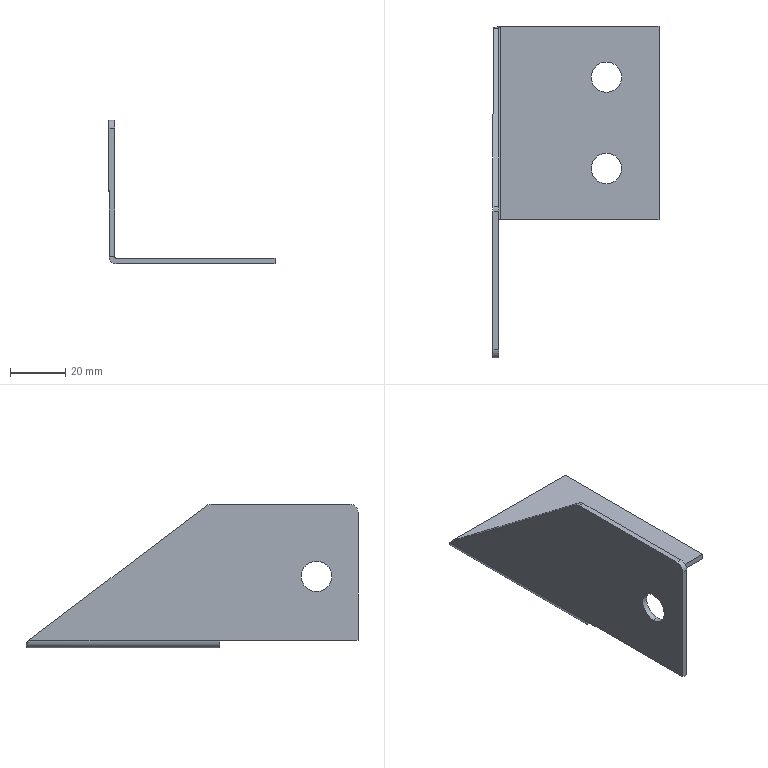Part | SolidWorks | features BaseBody 1 | 1 solid | 22 faces | box 60 x 120 x 52 mm | volume 16346 mm3 | plane 11 | cylinder 10 | spline 1 | commonest cylinder face diameters 11 x6 6 x2 1.473 x1 5.473 x1
STEP:
#1=CARTESIAN_POINT('',(-28.,-70.,18.368));
#2=VERTEX_POINT('',#1);
#3=CARTESIAN_POINT('',(-28.,-70.,29.368));
#4=VERTEX_POINT('',#3);
#5=CARTESIAN_POINT('',(-28.,-70.,23.868));
#6=DIRECTION('',(-1.,0.,0.));
#7=DIRECTION('',(0.,0.,1.));
#8=AXIS2_PLACEMENT_3D('',#5,#6,#7);
#9=CIRCLE('',#8,5.5);
#10=EDGE_CURVE('',#2,#4,#9,.T.);
#11=ORIENTED_EDGE('',*,*,#10,.F.);
#12=CARTESIAN_POINT('',(-30.,-70.,18.368));
#13=VERTEX_POINT('',#12);
#14=CARTESIAN_POINT('',(-20.,-70.,18.368));
#15=DIRECTION('',(-1.,0.,0.));
#16=VECTOR('',#15,1000.);
#17=LINE('',#14,#16);
#18=EDGE_CURVE('',#2,#13,#17,.T.);
#19=ORIENTED_EDGE('',*,*,#18,.T.);
#20=CARTESIAN_POINT('',(-30.,-70.,29.368));
#21=VERTEX_POINT('',#20);
#22=CARTESIAN_POINT('',(-30.,-70.,23.868));
#23=DIRECTION('',(1.,0.,0.));
#24=DIRECTION('',(0.,0.,1.));
#25=AXIS2_PLACEMENT_3D('',#22,#23,#24);
#26=CIRCLE('',#25,5.5);
#27=EDGE_CURVE('',#21,#13,#26,.T.);
#28=ORIENTED_EDGE('',*,*,#27,.F.);
#29=CARTESIAN_POINT('',(-20.,-70.,29.368));
#30=DIRECTION('',(-1.,0.,0.));
#31=VECTOR('',#30,1000.);
#32=LINE('',#29,#31);
#33=EDGE_CURVE('',#4,#21,#32,.T.);
#34=ORIENTED_EDGE('',*,*,#33,.F.);
#35=EDGE_LOOP('',(#11,#19,#28,#34));
#36=FACE_OUTER_BOUND('',#35,.T.);
#37=CARTESIAN_POINT('',(-20.,-70.,23.868));
#38=DIRECTION('',(-1.,0.,0.));
#39=DIRECTION('',(0.,0.,1.));
#40=AXIS2_PLACEMENT_3D('',#37,#38,#39);
#41=CYLINDRICAL_SURFACE('',#40,5.5);
#42=ADVANCED_FACE('',(#36),#41,.F.);
#43=CARTESIAN_POINT('',(5.5,16.5,-2.));
#44=VERTEX_POINT('',#43);
#45=CARTESIAN_POINT('',(16.5,16.5,-2.));
#46=VERTEX_POINT('',#45);
#47=CARTESIAN_POINT('',(11.,16.5,-2.));
#48=DIRECTION('',(0.,0.,1.));
#49=DIRECTION('',(1.,0.,0.));
#50=AXIS2_PLACEMENT_3D('',#47,#48,#49);
#51=CIRCLE('',#50,5.5);
#52=EDGE_CURVE('',#44,#46,#51,.T.);
#53=ORIENTED_EDGE('',*,*,#52,.F.);
#54=CARTESIAN_POINT('',(5.5,16.5,0.));
#55=VERTEX_POINT('',#54);
#56=CARTESIAN_POINT('',(5.5,16.5,-2.));
#57=DIRECTION('',(0.,0.,1.));
#58=VECTOR('',#57,1000.);
#59=LINE('',#56,#58);
#60=EDGE_CURVE('',#44,#55,#59,.T.);
#61=ORIENTED_EDGE('',*,*,#60,.T.);
#62=CARTESIAN_POINT('',(16.5,16.5,0.));
#63=VERTEX_POINT('',#62);
#64=CARTESIAN_POINT('',(11.,16.5,0.));
#65=DIRECTION('',(0.,0.,-1.));
#66=DIRECTION('',(1.,0.,0.));
#67=AXIS2_PLACEMENT_3D('',#64,#65,#66);
#68=CIRCLE('',#67,5.5);
#69=EDGE_CURVE('',#63,#55,#68,.T.);
#70=ORIENTED_EDGE('',*,*,#69,.F.);
#71=CARTESIAN_POINT('',(16.5,16.5,-2.));
#72=DIRECTION('',(0.,0.,1.));
#73=VECTOR('',#72,1000.);
#74=LINE('',#71,#73);
#75=EDGE_CURVE('',#46,#63,#74,.T.);
#76=ORIENTED_EDGE('',*,*,#75,.F.);
#77=EDGE_LOOP('',(#53,#61,#70,#76));
#78=FACE_OUTER_BOUND('',#77,.T.);
#79=CARTESIAN_POINT('',(11.,16.5,-2.));
#80=DIRECTION('',(0.,0.,1.));
#81=DIRECTION('',(1.,0.,0.));
#82=AXIS2_PLACEMENT_3D('',#79,#80,#81);
#83=CYLINDRICAL_SURFACE('',#82,5.5);
#84=ADVANCED_FACE('',(#78),#83,.F.);
#85=CARTESIAN_POINT('',(5.5,-16.5,-2.));
#86=VERTEX_POINT('',#85);
#87=CARTESIAN_POINT('',(16.5,-16.5,-2.));
#88=VERTEX_POINT('',#87);
#89=CARTESIAN_POINT('',(11.,-16.5,-2.));
#90=DIRECTION('',(0.,0.,1.));
#91=DIRECTION('',(1.,0.,0.));
#92=AXIS2_PLACEMENT_3D('',#89,#90,#91);
#93=CIRCLE('',#92,5.5);
#94=EDGE_CURVE('',#86,#88,#93,.T.);
#95=ORIENTED_EDGE('',*,*,#94,.F.);
#96=CARTESIAN_POINT('',(5.5,-16.5,0.));
#97=VERTEX_POINT('',#96);
#98=CARTESIAN_POINT('',(5.5,-16.5,-2.));
#99=DIRECTION('',(0.,0.,1.));
#100=VECTOR('',#99,1000.);
#101=LINE('',#98,#100);
#102=EDGE_CURVE('',#86,#97,#101,.T.);
#103=ORIENTED_EDGE('',*,*,#102,.T.);
#104=CARTESIAN_POINT('',(16.5,-16.5,0.));
#105=VERTEX_POINT('',#104);
#106=CARTESIAN_POINT('',(11.,-16.5,0.));
#107=DIRECTION('',(0.,0.,-1.));
#108=DIRECTION('',(1.,0.,0.));
#109=AXIS2_PLACEMENT_3D('',#106,#107,#108);
#110=CIRCLE('',#109,5.5);
#111=EDGE_CURVE('',#105,#97,#110,.T.);
#112=ORIENTED_EDGE('',*,*,#111,.F.);
#113=CARTESIAN_POINT('',(16.5,-16.5,-2.));
#114=DIRECTION('',(0.,0.,1.));
#115=VECTOR('',#114,1000.);
#116=LINE('',#113,#115);
#117=EDGE_CURVE('',#88,#105,#116,.T.);
#118=ORIENTED_EDGE('',*,*,#117,.F.);
#119=EDGE_LOOP('',(#95,#103,#112,#118));
#120=FACE_OUTER_BOUND('',#119,.T.);
#121=CARTESIAN_POINT('',(11.,-16.5,-2.));
#122=DIRECTION('',(0.,0.,1.));
#123=DIRECTION('',(1.,0.,0.));
#124=AXIS2_PLACEMENT_3D('',#121,#122,#123);
#125=CYLINDRICAL_SURFACE('',#124,5.5);
#126=ADVANCED_FACE('',(#120),#125,.F.);
#127=CARTESIAN_POINT('',(-30.,-82.,50.));
#128=VERTEX_POINT('',#127);
#129=CARTESIAN_POINT('',(-30.,-32.,50.));
#130=VERTEX_POINT('',#129);
#131=CARTESIAN_POINT('',(-30.,-32.,50.));
#132=DIRECTION('',(0.,1.,0.));
#133=VECTOR('',#132,1000.);
#134=LINE('',#131,#133);
#135=EDGE_CURVE('',#128,#130,#134,.T.);
#136=ORIENTED_EDGE('',*,*,#135,.T.);
#137=CARTESIAN_POINT('',(-30.,-30.188,49.391));
#138=VERTEX_POINT('',#137);
#139=CARTESIAN_POINT('',(-30.,-32.,47.));
#140=DIRECTION('',(-1.,0.,0.));
#141=DIRECTION('',(0.,0.,-1.));
#142=AXIS2_PLACEMENT_3D('',#139,#140,#141);
#143=CIRCLE('',#142,3.);
#144=EDGE_CURVE('',#130,#138,#143,.T.);
#145=ORIENTED_EDGE('',*,*,#144,.T.);
#146=CARTESIAN_POINT('',(-30.,34.028,0.7366));
#147=VERTEX_POINT('',#146);
#148=CARTESIAN_POINT('',(-30.,-30.188,49.391));
#149=DIRECTION('',(0.,0.7971,-0.6039));
#150=VECTOR('',#149,1000.);
#151=LINE('',#148,#150);
#152=EDGE_CURVE('',#138,#147,#151,.T.);
#153=ORIENTED_EDGE('',*,*,#152,.T.);
#154=CARTESIAN_POINT('',(-30.,-35.,0.7366));
#155=VERTEX_POINT('',#154);
#156=CARTESIAN_POINT('',(-30.,-32.,0.7366));
#157=DIRECTION('',(0.,-1.,0.));
#158=VECTOR('',#157,1000.);
#159=LINE('',#156,#158);
#160=EDGE_CURVE('',#147,#155,#159,.T.);
#161=ORIENTED_EDGE('',*,*,#160,.T.);
#162=CARTESIAN_POINT('',(-30.,-85.,0.7366));
#163=VERTEX_POINT('',#162);
#164=CARTESIAN_POINT('',(-30.,-32.,0.7366));
#165=DIRECTION('',(0.,-1.,0.));
#166=VECTOR('',#165,1000.);
#167=LINE('',#164,#166);
#168=EDGE_CURVE('',#155,#163,#167,.T.);
#169=ORIENTED_EDGE('',*,*,#168,.T.);
#170=CARTESIAN_POINT('',(-30.,-85.,47.));
#171=VERTEX_POINT('',#170);
#172=CARTESIAN_POINT('',(-30.,-85.,47.));
#173=DIRECTION('',(0.,0.,1.));
#174=VECTOR('',#173,1000.);
#175=LINE('',#172,#174);
#176=EDGE_CURVE('',#163,#171,#175,.T.);
#177=ORIENTED_EDGE('',*,*,#176,.T.);
#178=CARTESIAN_POINT('',(-30.,-82.,47.));
#179=DIRECTION('',(-1.,0.,0.));
#180=DIRECTION('',(0.,0.,-1.));
#181=AXIS2_PLACEMENT_3D('',#178,#179,#180);
#182=CIRCLE('',#181,3.);
#183=EDGE_CURVE('',#171,#128,#182,.T.);
#184=ORIENTED_EDGE('',*,*,#183,.T.);
#185=EDGE_LOOP('',(#136,#145,#153,#161,#169,#177,#184));
#186=FACE_OUTER_BOUND('',#185,.T.);
#187=ORIENTED_EDGE('',*,*,#27,.T.);
#188=CARTESIAN_POINT('',(-30.,-70.,23.868));
#189=DIRECTION('',(1.,0.,0.));
#190=DIRECTION('',(0.,0.,1.));
#191=AXIS2_PLACEMENT_3D('',#188,#189,#190);
#192=CIRCLE('',#191,5.5);
#193=EDGE_CURVE('',#13,#21,#192,.T.);
#194=ORIENTED_EDGE('',*,*,#193,.T.);
#195=EDGE_LOOP('',(#187,#194));
#196=FACE_BOUND('',#195,.T.);
#197=CARTESIAN_POINT('',(-30.,-32.,47.));
#198=DIRECTION('',(-1.,0.,0.));
#199=DIRECTION('',(0.,0.,1.));
#200=AXIS2_PLACEMENT_3D('',#197,#198,#199);
#201=PLANE('',#200);
#202=ADVANCED_FACE('',(#186,#196),#201,.T.);
#203=ORIENTED_EDGE('',*,*,#144,.F.);
#204=CARTESIAN_POINT('',(-28.,-32.,50.));
#205=VERTEX_POINT('',#204);
#206=CARTESIAN_POINT('',(-30.,-32.,50.));
#207=DIRECTION('',(1.,0.,0.));
#208=VECTOR('',#207,1000.);
#209=LINE('',#206,#208);
#210=EDGE_CURVE('',#130,#205,#209,.T.);
#211=ORIENTED_EDGE('',*,*,#210,.T.);
#212=CARTESIAN_POINT('',(-28.,-30.188,49.391));
#213=VERTEX_POINT('',#212);
#214=CARTESIAN_POINT('',(-28.,-32.,47.));
#215=DIRECTION('',(-1.,0.,0.));
#216=DIRECTION('',(0.,0.,-1.));
#217=AXIS2_PLACEMENT_3D('',#214,#215,#216);
#218=CIRCLE('',#217,3.);
#219=EDGE_CURVE('',#205,#213,#218,.T.);
#220=ORIENTED_EDGE('',*,*,#219,.T.);
#221=CARTESIAN_POINT('',(-30.,-30.188,49.391));
#222=DIRECTION('',(-1.,0.,0.));
#223=VECTOR('',#222,1000.);
#224=LINE('',#221,#223);
#225=EDGE_CURVE('',#213,#138,#224,.T.);
#226=ORIENTED_EDGE('',*,*,#225,.T.);
#227=EDGE_LOOP('',(#203,#211,#220,#226));
#228=FACE_OUTER_BOUND('',#227,.T.);
#229=CARTESIAN_POINT('',(-30.,-32.,47.));
#230=DIRECTION('',(1.,0.,0.));
#231=DIRECTION('',(0.,0.,-1.));
#232=AXIS2_PLACEMENT_3D('',#229,#230,#231);
#233=CYLINDRICAL_SURFACE('',#232,3.);
#234=ADVANCED_FACE('',(#228),#233,.T.);
#235=ORIENTED_EDGE('',*,*,#210,.F.);
#236=ORIENTED_EDGE('',*,*,#135,.F.);
#237=CARTESIAN_POINT('',(-28.,-82.,50.));
#238=VERTEX_POINT('',#237);
#239=CARTESIAN_POINT('',(-30.,-82.,50.));
#240=DIRECTION('',(-1.,0.,0.));
#241=VECTOR('',#240,1000.);
#242=LINE('',#239,#241);
#243=EDGE_CURVE('',#238,#128,#242,.T.);
#244=ORIENTED_EDGE('',*,*,#243,.F.);
#245=CARTESIAN_POINT('',(-28.,-32.,50.));
#246=DIRECTION('',(0.,-1.,0.));
#247=VECTOR('',#246,1000.);
#248=LINE('',#245,#247);
#249=EDGE_CURVE('',#205,#238,#248,.T.);
#250=ORIENTED_EDGE('',*,*,#249,.F.);
#251=EDGE_LOOP('',(#235,#236,#244,#250));
#252=FACE_OUTER_BOUND('',#251,.T.);
#253=CARTESIAN_POINT('',(-30.,-32.,50.));
#254=DIRECTION('',(0.,0.,-1.));
#255=DIRECTION('',(-1.,0.,0.));
#256=AXIS2_PLACEMENT_3D('',#253,#254,#255);
#257=PLANE('',#256);
#258=ADVANCED_FACE('',(#252),#257,.F.);
#259=ORIENTED_EDGE('',*,*,#183,.F.);
#260=CARTESIAN_POINT('',(-28.,-85.,47.));
#261=VERTEX_POINT('',#260);
#262=CARTESIAN_POINT('',(-30.,-85.,47.));
#263=DIRECTION('',(1.,0.,0.));
#264=VECTOR('',#263,1000.);
#265=LINE('',#262,#264);
#266=EDGE_CURVE('',#171,#261,#265,.T.);
#267=ORIENTED_EDGE('',*,*,#266,.T.);
#268=CARTESIAN_POINT('',(-28.,-82.,47.));
#269=DIRECTION('',(-1.,0.,0.));
#270=DIRECTION('',(0.,0.,-1.));
#271=AXIS2_PLACEMENT_3D('',#268,#269,#270);
#272=CIRCLE('',#271,3.);
#273=EDGE_CURVE('',#261,#238,#272,.T.);
#274=ORIENTED_EDGE('',*,*,#273,.T.);
#275=ORIENTED_EDGE('',*,*,#243,.T.);
#276=EDGE_LOOP('',(#259,#267,#274,#275));
#277=FACE_OUTER_BOUND('',#276,.T.);
#278=CARTESIAN_POINT('',(-30.,-82.,47.));
#279=DIRECTION('',(1.,0.,0.));
#280=DIRECTION('',(0.,0.,-1.));
#281=AXIS2_PLACEMENT_3D('',#278,#279,#280);
#282=CYLINDRICAL_SURFACE('',#281,3.);
#283=ADVANCED_FACE('',(#277),#282,.T.);
#284=CARTESIAN_POINT('',(-28.,-85.,0.7366));
#285=VERTEX_POINT('',#284);
#286=CARTESIAN_POINT('',(-28.,-85.,47.));
#287=DIRECTION('',(0.,0.,-1.));
#288=VECTOR('',#287,1000.);
#289=LINE('',#286,#288);
#290=EDGE_CURVE('',#261,#285,#289,.T.);
#291=ORIENTED_EDGE('',*,*,#290,.F.);
#292=ORIENTED_EDGE('',*,*,#266,.F.);
#293=ORIENTED_EDGE('',*,*,#176,.F.);
#294=CARTESIAN_POINT('',(-30.,-85.,0.7366));
#295=DIRECTION('',(-1.,0.,0.));
#296=VECTOR('',#295,1000.);
#297=LINE('',#294,#296);
#298=EDGE_CURVE('',#285,#163,#297,.T.);
#299=ORIENTED_EDGE('',*,*,#298,.F.);
#300=EDGE_LOOP('',(#291,#292,#293,#299));
#301=FACE_OUTER_BOUND('',#300,.T.);
#302=CARTESIAN_POINT('',(-30.,-85.,47.));
#303=DIRECTION('',(0.,1.,0.));
#304=DIRECTION('',(0.,0.,1.));
#305=AXIS2_PLACEMENT_3D('',#302,#303,#304);
#306=PLANE('',#305);
#307=ADVANCED_FACE('',(#301),#306,.F.);
#308=ORIENTED_EDGE('',*,*,#298,.T.);
#309=ORIENTED_EDGE('',*,*,#168,.F.);
#310=CARTESIAN_POINT('',(-28.,-35.,0.7366));
#311=VERTEX_POINT('',#310);
#312=CARTESIAN_POINT('',(-28.,-35.,0.7366));
#313=DIRECTION('',(1.,0.,0.));
#314=VECTOR('',#313,1000.);
#315=LINE('',#312,#314);
#316=EDGE_CURVE('',#155,#311,#315,.T.);
#317=ORIENTED_EDGE('',*,*,#316,.T.);
#318=CARTESIAN_POINT('',(-28.,34.028,0.7366));
#319=DIRECTION('',(0.,-1.,0.));
#320=VECTOR('',#319,1000.);
#321=LINE('',#318,#320);
#322=EDGE_CURVE('',#311,#285,#321,.T.);
#323=ORIENTED_EDGE('',*,*,#322,.T.);
#324=EDGE_LOOP('',(#308,#309,#317,#323));
#325=FACE_OUTER_BOUND('',#324,.T.);
#326=CARTESIAN_POINT('',(-28.,34.028,0.7366));
#327=DIRECTION('',(0.,0.,-1.));
#328=DIRECTION('',(-1.,0.,0.));
#329=AXIS2_PLACEMENT_3D('',#326,#327,#328);
#330=PLANE('',#329);
#331=ADVANCED_FACE('',(#325),#330,.T.);
#332=ORIENTED_EDGE('',*,*,#160,.F.);
#333=CARTESIAN_POINT('',(-27.263,35.,-2.));
#334=VERTEX_POINT('',#333);
#335=CARTESIAN_POINT('',(-30.,34.028,0.7366));
#336=CARTESIAN_POINT('',(-30.,34.11,0.3751));
#337=CARTESIAN_POINT('',(-29.93,34.189,0.02414));
#338=CARTESIAN_POINT('',(-29.723,34.311,-0.4757));
#339=CARTESIAN_POINT('',(-29.639,34.351,-0.6331));
#340=CARTESIAN_POINT('',(-29.441,34.432,-0.9298));
#341=CARTESIAN_POINT('',(-29.326,34.473,-1.071));
#342=CARTESIAN_POINT('',(-29.073,34.554,-1.324));
#343=CARTESIAN_POINT('',(-28.935,34.594,-1.437));
#344=CARTESIAN_POINT('',(-28.638,34.675,-1.636));
#345=CARTESIAN_POINT('',(-28.478,34.716,-1.722));
#346=CARTESIAN_POINT('',(-28.148,34.797,-1.859));
#347=CARTESIAN_POINT('',(-27.977,34.837,-1.911));
#348=CARTESIAN_POINT('',(-27.625,34.918,-1.982));
#349=CARTESIAN_POINT('',(-27.444,34.959,-2.));
#350=CARTESIAN_POINT('',(-27.263,35.,-2.));
#351=B_SPLINE_CURVE_WITH_KNOTS('',3,(#335,#336,#337,#338,#339,#340,#341,#342,#343,#344,#345,#346,#347,#348,#349,#350),.UNSPECIFIED.,.F.,.F.,(4,2,2,2,2,2,2,4),(0.,0.001093,0.00164,0.002187,0.002734,0.00328,0.003827,0.004374),.UNSPECIFIED.);
#352=EDGE_CURVE('',#147,#334,#351,.T.);
#353=ORIENTED_EDGE('',*,*,#352,.T.);
#354=CARTESIAN_POINT('',(-27.263,-35.,-2.));
#355=VERTEX_POINT('',#354);
#356=CARTESIAN_POINT('',(-27.263,-35.,-2.));
#357=DIRECTION('',(0.,-1.,0.));
#358=VECTOR('',#357,1000.);
#359=LINE('',#356,#358);
#360=EDGE_CURVE('',#334,#355,#359,.T.);
#361=ORIENTED_EDGE('',*,*,#360,.T.);
#362=CARTESIAN_POINT('',(-27.263,-35.,0.7366));
#363=DIRECTION('',(0.,1.,0.));
#364=DIRECTION('',(0.,0.,-1.));
#365=AXIS2_PLACEMENT_3D('',#362,#363,#364);
#366=CIRCLE('',#365,2.737);
#367=EDGE_CURVE('',#355,#155,#366,.T.);
#368=ORIENTED_EDGE('',*,*,#367,.T.);
#369=EDGE_LOOP('',(#332,#353,#361,#368));
#370=FACE_OUTER_BOUND('',#369,.T.);
#371=CARTESIAN_POINT('',(-27.263,-35.,0.7366));
#372=DIRECTION('',(0.,-1.,0.));
#373=DIRECTION('',(0.,0.,-1.));
#374=AXIS2_PLACEMENT_3D('',#371,#372,#373);
#375=CYLINDRICAL_SURFACE('',#374,2.737);
#376=ADVANCED_FACE('',(#370),#375,.T.);
#377=ORIENTED_EDGE('',*,*,#152,.F.);
#378=ORIENTED_EDGE('',*,*,#225,.F.);
#379=CARTESIAN_POINT('',(-28.,34.028,0.7366));
#380=VERTEX_POINT('',#379);
#381=CARTESIAN_POINT('',(-28.,35.,0.));
#382=DIRECTION('',(0.,-0.7971,0.6039));
#383=VECTOR('',#382,1000.);
#384=LINE('',#381,#383);
#385=EDGE_CURVE('',#380,#213,#384,.T.);
#386=ORIENTED_EDGE('',*,*,#385,.F.);
#387=CARTESIAN_POINT('',(-30.,34.028,0.7366));
#388=DIRECTION('',(1.,0.,0.));
#389=VECTOR('',#388,1000.);
#390=LINE('',#387,#389);
#391=EDGE_CURVE('',#147,#380,#390,.T.);
#392=ORIENTED_EDGE('',*,*,#391,.F.);
#393=EDGE_LOOP('',(#377,#378,#386,#392));
#394=FACE_OUTER_BOUND('',#393,.T.);
#395=CARTESIAN_POINT('',(-30.,35.,0.));
#396=DIRECTION('',(0.,-0.6039,-0.7971));
#397=DIRECTION('',(0.,0.7971,-0.6039));
#398=AXIS2_PLACEMENT_3D('',#395,#396,#397);
#399=PLANE('',#398);
#400=ADVANCED_FACE('',(#394),#399,.F.);
#401=ORIENTED_EDGE('',*,*,#18,.F.);
#402=CARTESIAN_POINT('',(-28.,-70.,23.868));
#403=DIRECTION('',(-1.,0.,0.));
#404=DIRECTION('',(0.,0.,1.));
#405=AXIS2_PLACEMENT_3D('',#402,#403,#404);
#406=CIRCLE('',#405,5.5);
#407=EDGE_CURVE('',#4,#2,#406,.T.);
#408=ORIENTED_EDGE('',*,*,#407,.F.);
#409=ORIENTED_EDGE('',*,*,#33,.T.);
#410=ORIENTED_EDGE('',*,*,#193,.F.);
#411=EDGE_LOOP('',(#401,#408,#409,#410));
#412=FACE_OUTER_BOUND('',#411,.T.);
#413=CARTESIAN_POINT('',(-20.,-70.,23.868));
#414=DIRECTION('',(-1.,0.,0.));
#415=DIRECTION('',(0.,0.,1.));
#416=AXIS2_PLACEMENT_3D('',#413,#414,#415);
#417=CYLINDRICAL_SURFACE('',#416,5.5);
#418=ADVANCED_FACE('',(#412),#417,.F.);
#419=ORIENTED_EDGE('',*,*,#385,.T.);
#420=ORIENTED_EDGE('',*,*,#219,.F.);
#421=ORIENTED_EDGE('',*,*,#249,.T.);
#422=ORIENTED_EDGE('',*,*,#273,.F.);
#423=ORIENTED_EDGE('',*,*,#290,.T.);
#424=ORIENTED_EDGE('',*,*,#322,.F.);
#425=CARTESIAN_POINT('',(-28.,-32.,0.7366));
#426=DIRECTION('',(0.,-1.,0.));
#427=VECTOR('',#426,1000.);
#428=LINE('',#425,#427);
#429=EDGE_CURVE('',#380,#311,#428,.T.);
#430=ORIENTED_EDGE('',*,*,#429,.F.);
#431=EDGE_LOOP('',(#419,#420,#421,#422,#423,#424,#430));
#432=FACE_OUTER_BOUND('',#431,.T.);
#433=ORIENTED_EDGE('',*,*,#407,.T.);
#434=ORIENTED_EDGE('',*,*,#10,.T.);
#435=EDGE_LOOP('',(#433,#434));
#436=FACE_BOUND('',#435,.T.);
#437=CARTESIAN_POINT('',(-28.,-32.,47.));
#438=DIRECTION('',(-1.,0.,0.));
#439=DIRECTION('',(0.,0.,1.));
#440=AXIS2_PLACEMENT_3D('',#437,#438,#439);
#441=PLANE('',#440);
#442=ADVANCED_FACE('',(#432,#436),#441,.F.);
#443=ORIENTED_EDGE('',*,*,#316,.F.);
#444=ORIENTED_EDGE('',*,*,#367,.F.);
#445=CARTESIAN_POINT('',(30.,-35.,-2.));
#446=VERTEX_POINT('',#445);
#447=CARTESIAN_POINT('',(0.,-35.,-2.));
#448=DIRECTION('',(-1.,0.,0.));
#449=VECTOR('',#448,1000.);
#450=LINE('',#447,#449);
#451=EDGE_CURVE('',#446,#355,#450,.T.);
#452=ORIENTED_EDGE('',*,*,#451,.F.);
#453=CARTESIAN_POINT('',(30.,-35.,0.));
#454=VERTEX_POINT('',#453);
#455=CARTESIAN_POINT('',(30.,-35.,-2.));
#456=DIRECTION('',(0.,0.,1.));
#457=VECTOR('',#456,1000.);
#458=LINE('',#455,#457);
#459=EDGE_CURVE('',#446,#454,#458,.T.);
#460=ORIENTED_EDGE('',*,*,#459,.T.);
#461=CARTESIAN_POINT('',(-27.263,-35.,0.));
#462=VERTEX_POINT('',#461);
#463=CARTESIAN_POINT('',(-30.,-35.,0.));
#464=DIRECTION('',(-1.,0.,0.));
#465=VECTOR('',#464,1000.);
#466=LINE('',#463,#465);
#467=EDGE_CURVE('',#454,#462,#466,.T.);
#468=ORIENTED_EDGE('',*,*,#467,.T.);
#469=CARTESIAN_POINT('',(-27.263,-35.,0.7366));
#470=DIRECTION('',(0.,-1.,0.));
#471=DIRECTION('',(0.,0.,-1.));
#472=AXIS2_PLACEMENT_3D('',#469,#470,#471);
#473=CIRCLE('',#472,0.7366);
#474=EDGE_CURVE('',#311,#462,#473,.T.);
#475=ORIENTED_EDGE('',*,*,#474,.F.);
#476=EDGE_LOOP('',(#443,#444,#452,#460,#468,#475));
#477=FACE_OUTER_BOUND('',#476,.T.);
#478=CARTESIAN_POINT('',(-27.263,-35.,0.7366));
#479=DIRECTION('',(0.,1.,0.));
#480=DIRECTION('',(0.,0.,1.));
#481=AXIS2_PLACEMENT_3D('',#478,#479,#480);
#482=PLANE('',#481);
#483=ADVANCED_FACE('',(#477),#482,.F.);
#484=CARTESIAN_POINT('',(-27.263,35.,0.));
#485=VERTEX_POINT('',#484);
#486=CARTESIAN_POINT('',(-27.263,35.,0.));
#487=CARTESIAN_POINT('',(-27.458,34.837,0.));
#488=CARTESIAN_POINT('',(-27.647,34.677,0.07876));
#489=CARTESIAN_POINT('',(-27.921,34.352,0.3521));
#490=CARTESIAN_POINT('',(-28.,34.191,0.5422));
#491=CARTESIAN_POINT('',(-28.,34.028,0.7366));
#492=B_SPLINE_CURVE_WITH_KNOTS('',3,(#486,#487,#488,#489,#490,#491),.UNSPECIFIED.,.F.,.F.,(4,2,4),(0.,0.0007533,0.001507),.UNSPECIFIED.);
#493=EDGE_CURVE('',#485,#380,#492,.T.);
#494=ORIENTED_EDGE('',*,*,#493,.F.);
#495=CARTESIAN_POINT('',(-27.263,35.,-0.9999));
#496=DIRECTION('',(0.,0.,1.));
#497=VECTOR('',#496,1000.);
#498=LINE('',#495,#497);
#499=EDGE_CURVE('',#334,#485,#498,.T.);
#500=ORIENTED_EDGE('',*,*,#499,.F.);
#501=ORIENTED_EDGE('',*,*,#352,.F.);
#502=ORIENTED_EDGE('',*,*,#391,.T.);
#503=EDGE_LOOP('',(#494,#500,#501,#502));
#504=FACE_OUTER_BOUND('',#503,.T.);
#505=CARTESIAN_POINT('',(-27.263,35.,-2.02));
#506=CARTESIAN_POINT('',(-27.624,34.919,-2.02));
#507=CARTESIAN_POINT('',(-27.985,34.838,-1.948));
#508=CARTESIAN_POINT('',(-28.652,34.676,-1.672));
#509=CARTESIAN_POINT('',(-28.957,34.595,-1.468));
#510=CARTESIAN_POINT('',(-29.468,34.433,-0.9575));
#511=CARTESIAN_POINT('',(-29.672,34.352,-0.6517));
#512=CARTESIAN_POINT('',(-29.948,34.19,0.01507));
#513=CARTESIAN_POINT('',(-30.02,34.109,0.3757));
#514=CARTESIAN_POINT('',(-30.02,34.028,0.7366));
#515=CARTESIAN_POINT('',(-27.263,35.,-2.));
#516=CARTESIAN_POINT('',(-27.622,34.919,-2.));
#517=CARTESIAN_POINT('',(-27.98,34.838,-1.929));
#518=CARTESIAN_POINT('',(-28.642,34.676,-1.655));
#519=CARTESIAN_POINT('',(-28.945,34.595,-1.452));
#520=CARTESIAN_POINT('',(-29.452,34.433,-0.9452));
#521=CARTESIAN_POINT('',(-29.655,34.352,-0.6416));
#522=CARTESIAN_POINT('',(-29.929,34.19,0.0203));
#523=CARTESIAN_POINT('',(-30.,34.109,0.3783));
#524=CARTESIAN_POINT('',(-30.,34.028,0.7366));
#525=CARTESIAN_POINT('',(-27.263,35.,0.));
#526=CARTESIAN_POINT('',(-27.36,34.919,0.));
#527=CARTESIAN_POINT('',(-27.456,34.838,0.01917));
#528=CARTESIAN_POINT('',(-27.634,34.676,0.09297));
#529=CARTESIAN_POINT('',(-27.716,34.595,0.1476));
#530=CARTESIAN_POINT('',(-27.852,34.433,0.2839));
#531=CARTESIAN_POINT('',(-27.907,34.352,0.3656));
#532=CARTESIAN_POINT('',(-27.981,34.19,0.5438));
#533=CARTESIAN_POINT('',(-28.,34.109,0.6402));
#534=CARTESIAN_POINT('',(-28.,34.028,0.7366));
#535=CARTESIAN_POINT('',(-27.263,35.,0.0202));
#536=CARTESIAN_POINT('',(-27.357,34.919,0.0202));
#537=CARTESIAN_POINT('',(-27.451,34.838,0.03885));
#538=CARTESIAN_POINT('',(-27.624,34.676,0.1106));
#539=CARTESIAN_POINT('',(-27.704,34.595,0.1637));
#540=CARTESIAN_POINT('',(-27.836,34.433,0.2963));
#541=CARTESIAN_POINT('',(-27.889,34.352,0.3758));
#542=CARTESIAN_POINT('',(-27.961,34.19,0.5491));
#543=CARTESIAN_POINT('',(-27.98,34.109,0.6428));
#544=CARTESIAN_POINT('',(-27.98,34.028,0.7366));
#545=B_SPLINE_SURFACE_WITH_KNOTS('',1,3,((#505,#506,#507,#508,#509,#510,#511,#512,#513,#514),(#515,#516,#517,#518,#519,#520,#521,#522,#523,#524),(#525,#526,#527,#528,#529,#530,#531,#532,#533,#534),(#535,#536,#537,#538,#539,#540,#541,#542,#543,#544)),.UNSPECIFIED.,.F.,.F.,.F.,(2,1,1,2),(4,2,2,2,4),(-0.01,0.,1.,1.01),(0.,0.25,0.5,0.75,1.),.UNSPECIFIED.);
#546=ADVANCED_FACE('',(#504),#545,.F.);
#547=CARTESIAN_POINT('',(30.,35.,-2.));
#548=VERTEX_POINT('',#547);
#549=CARTESIAN_POINT('',(0.,35.,-2.));
#550=DIRECTION('',(1.,0.,0.));
#551=VECTOR('',#550,1000.);
#552=LINE('',#549,#551);
#553=EDGE_CURVE('',#334,#548,#552,.T.);
#554=ORIENTED_EDGE('',*,*,#553,.T.);
#555=CARTESIAN_POINT('',(30.,0.,-2.));
#556=DIRECTION('',(0.,-1.,0.));
#557=VECTOR('',#556,1000.);
#558=LINE('',#555,#557);
#559=EDGE_CURVE('',#548,#446,#558,.T.);
#560=ORIENTED_EDGE('',*,*,#559,.T.);
#561=ORIENTED_EDGE('',*,*,#451,.T.);
#562=ORIENTED_EDGE('',*,*,#360,.F.);
#563=EDGE_LOOP('',(#554,#560,#561,#562));
#564=FACE_OUTER_BOUND('',#563,.T.);
#565=CARTESIAN_POINT('',(11.,16.5,-2.));
#566=DIRECTION('',(0.,0.,1.));
#567=DIRECTION('',(1.,0.,0.));
#568=AXIS2_PLACEMENT_3D('',#565,#566,#567);
#569=CIRCLE('',#568,5.5);
#570=EDGE_CURVE('',#46,#44,#569,.T.);
#571=ORIENTED_EDGE('',*,*,#570,.T.);
#572=ORIENTED_EDGE('',*,*,#52,.T.);
#573=EDGE_LOOP('',(#571,#572));
#574=FACE_BOUND('',#573,.T.);
#575=CARTESIAN_POINT('',(11.,-16.5,-2.));
#576=DIRECTION('',(0.,0.,1.));
#577=DIRECTION('',(1.,0.,0.));
#578=AXIS2_PLACEMENT_3D('',#575,#576,#577);
#579=CIRCLE('',#578,5.5);
#580=EDGE_CURVE('',#88,#86,#579,.T.);
#581=ORIENTED_EDGE('',*,*,#580,.T.);
#582=ORIENTED_EDGE('',*,*,#94,.T.);
#583=EDGE_LOOP('',(#581,#582));
#584=FACE_BOUND('',#583,.T.);
#585=CARTESIAN_POINT('',(0.,0.,-2.));
#586=DIRECTION('',(0.,0.,-1.));
#587=DIRECTION('',(-1.,0.,0.));
#588=AXIS2_PLACEMENT_3D('',#585,#586,#587);
#589=PLANE('',#588);
#590=ADVANCED_FACE('',(#564,#574,#584),#589,.T.);
#591=ORIENTED_EDGE('',*,*,#493,.T.);
#592=ORIENTED_EDGE('',*,*,#429,.T.);
#593=ORIENTED_EDGE('',*,*,#474,.T.);
#594=CARTESIAN_POINT('',(-27.263,-35.,0.));
#595=DIRECTION('',(0.,-1.,0.));
#596=VECTOR('',#595,1000.);
#597=LINE('',#594,#596);
#598=EDGE_CURVE('',#485,#462,#597,.T.);
#599=ORIENTED_EDGE('',*,*,#598,.F.);
#600=EDGE_LOOP('',(#591,#592,#593,#599));
#601=FACE_OUTER_BOUND('',#600,.T.);
#602=CARTESIAN_POINT('',(-27.263,-35.,0.7366));
#603=DIRECTION('',(0.,-1.,0.));
#604=DIRECTION('',(0.,0.,-1.));
#605=AXIS2_PLACEMENT_3D('',#602,#603,#604);
#606=CYLINDRICAL_SURFACE('',#605,0.7366);
#607=ADVANCED_FACE('',(#601),#606,.F.);
#608=CARTESIAN_POINT('',(30.,35.,0.));
#609=VERTEX_POINT('',#608);
#610=CARTESIAN_POINT('',(30.,35.,-2.));
#611=DIRECTION('',(0.,0.,-1.));
#612=VECTOR('',#611,1000.);
#613=LINE('',#610,#612);
#614=EDGE_CURVE('',#609,#548,#613,.T.);
#615=ORIENTED_EDGE('',*,*,#614,.T.);
#616=ORIENTED_EDGE('',*,*,#553,.F.);
#617=ORIENTED_EDGE('',*,*,#499,.T.);
#618=CARTESIAN_POINT('',(-30.,35.,0.));
#619=DIRECTION('',(1.,0.,0.));
#620=VECTOR('',#619,1000.);
#621=LINE('',#618,#620);
#622=EDGE_CURVE('',#485,#609,#621,.T.);
#623=ORIENTED_EDGE('',*,*,#622,.T.);
#624=EDGE_LOOP('',(#615,#616,#617,#623));
#625=FACE_OUTER_BOUND('',#624,.T.);
#626=CARTESIAN_POINT('',(-30.,35.,-2.));
#627=DIRECTION('',(0.,1.,0.));
#628=DIRECTION('',(0.,0.,1.));
#629=AXIS2_PLACEMENT_3D('',#626,#627,#628);
#630=PLANE('',#629);
#631=ADVANCED_FACE('',(#625),#630,.T.);
#632=ORIENTED_EDGE('',*,*,#559,.F.);
#633=ORIENTED_EDGE('',*,*,#614,.F.);
#634=CARTESIAN_POINT('',(30.,-35.,0.));
#635=DIRECTION('',(0.,-1.,0.));
#636=VECTOR('',#635,1000.);
#637=LINE('',#634,#636);
#638=EDGE_CURVE('',#609,#454,#637,.T.);
#639=ORIENTED_EDGE('',*,*,#638,.T.);
#640=ORIENTED_EDGE('',*,*,#459,.F.);
#641=EDGE_LOOP('',(#632,#633,#639,#640));
#642=FACE_OUTER_BOUND('',#641,.T.);
#643=CARTESIAN_POINT('',(30.,-35.,-2.));
#644=DIRECTION('',(1.,0.,0.));
#645=DIRECTION('',(0.,0.,-1.));
#646=AXIS2_PLACEMENT_3D('',#643,#644,#645);
#647=PLANE('',#646);
#648=ADVANCED_FACE('',(#642),#647,.T.);
#649=ORIENTED_EDGE('',*,*,#60,.F.);
#650=ORIENTED_EDGE('',*,*,#570,.F.);
#651=ORIENTED_EDGE('',*,*,#75,.T.);
#652=CARTESIAN_POINT('',(11.,16.5,0.));
#653=DIRECTION('',(0.,0.,-1.));
#654=DIRECTION('',(1.,0.,0.));
#655=AXIS2_PLACEMENT_3D('',#652,#653,#654);
#656=CIRCLE('',#655,5.5);
#657=EDGE_CURVE('',#55,#63,#656,.T.);
#658=ORIENTED_EDGE('',*,*,#657,.F.);
#659=EDGE_LOOP('',(#649,#650,#651,#658));
#660=FACE_OUTER_BOUND('',#659,.T.);
#661=CARTESIAN_POINT('',(11.,16.5,-2.));
#662=DIRECTION('',(0.,0.,1.));
#663=DIRECTION('',(1.,0.,0.));
#664=AXIS2_PLACEMENT_3D('',#661,#662,#663);
#665=CYLINDRICAL_SURFACE('',#664,5.5);
#666=ADVANCED_FACE('',(#660),#665,.F.);
#667=ORIENTED_EDGE('',*,*,#102,.F.);
#668=ORIENTED_EDGE('',*,*,#580,.F.);
#669=ORIENTED_EDGE('',*,*,#117,.T.);
#670=CARTESIAN_POINT('',(11.,-16.5,0.));
#671=DIRECTION('',(0.,0.,-1.));
#672=DIRECTION('',(1.,0.,0.));
#673=AXIS2_PLACEMENT_3D('',#670,#671,#672);
#674=CIRCLE('',#673,5.5);
#675=EDGE_CURVE('',#97,#105,#674,.T.);
#676=ORIENTED_EDGE('',*,*,#675,.F.);
#677=EDGE_LOOP('',(#667,#668,#669,#676));
#678=FACE_OUTER_BOUND('',#677,.T.);
#679=CARTESIAN_POINT('',(11.,-16.5,-2.));
#680=DIRECTION('',(0.,0.,1.));
#681=DIRECTION('',(1.,0.,0.));
#682=AXIS2_PLACEMENT_3D('',#679,#680,#681);
#683=CYLINDRICAL_SURFACE('',#682,5.5);
#684=ADVANCED_FACE('',(#678),#683,.F.);
#685=ORIENTED_EDGE('',*,*,#467,.F.);
#686=ORIENTED_EDGE('',*,*,#638,.F.);
#687=ORIENTED_EDGE('',*,*,#622,.F.);
#688=ORIENTED_EDGE('',*,*,#598,.T.);
#689=EDGE_LOOP('',(#685,#686,#687,#688));
#690=FACE_OUTER_BOUND('',#689,.T.);
#691=ORIENTED_EDGE('',*,*,#111,.T.);
#692=ORIENTED_EDGE('',*,*,#675,.T.);
#693=EDGE_LOOP('',(#691,#692));
#694=FACE_BOUND('',#693,.T.);
#695=ORIENTED_EDGE('',*,*,#69,.T.);
#696=ORIENTED_EDGE('',*,*,#657,.T.);
#697=EDGE_LOOP('',(#695,#696));
#698=FACE_BOUND('',#697,.T.);
#699=CARTESIAN_POINT('',(0.,0.,0.));
#700=DIRECTION('',(0.,0.,-1.));
#701=DIRECTION('',(-1.,0.,0.));
#702=AXIS2_PLACEMENT_3D('',#699,#700,#701);
#703=PLANE('',#702);
#704=ADVANCED_FACE('',(#690,#694,#698),#703,.F.);
#705=CLOSED_SHELL('',(#42,#84,#126,#202,#234,#258,#283,#307,#331,#376,#400,#418,#442,#483,#546,#590,#607,#631,#648,#666,#684,#704));
#706=MANIFOLD_SOLID_BREP('',#705);
#707=CARTESIAN_POINT('',(0.,0.,0.));
#708=DIRECTION('',(0.,0.,1.));
#709=DIRECTION('',(1.,0.,0.));
#710=AXIS2_PLACEMENT_3D('',#707,#708,#709);
#711=(LENGTH_UNIT()NAMED_UNIT(*)SI_UNIT(.MILLI.,.METRE.));
#712=UNCERTAINTY_MEASURE_WITH_UNIT(LENGTH_MEASURE(0.00001),#711,'','');
#713=(NAMED_UNIT(*)PLANE_ANGLE_UNIT()SI_UNIT($,.RADIAN.));
#714=(NAMED_UNIT(*)SI_UNIT($,.STERADIAN.)SOLID_ANGLE_UNIT());
#715=(GEOMETRIC_REPRESENTATION_CONTEXT(3)GLOBAL_UNCERTAINTY_ASSIGNED_CONTEXT((#712))GLOBAL_UNIT_ASSIGNED_CONTEXT((#711,#713,#714))REPRESENTATION_CONTEXT('',''));
#716=ADVANCED_BREP_SHAPE_REPRESENTATION('',(#706,#710),#715);